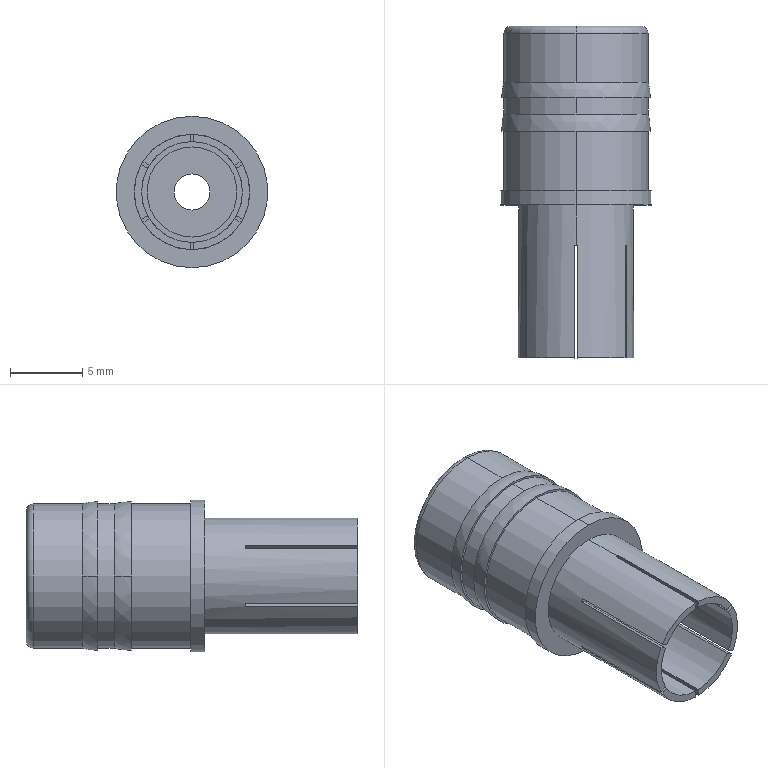Part | SolidWorks | features CirPattern 1, Fillet 1, ICE 1, Revolution 1 | 1 solid | 53 faces | box 10.5 x 23 x 10.5 mm | volume 736.39 mm3 | plane 31 | cylinder 16 | spline 4 | torus 2 | commonest cylinder face diameters 10 x6 2.5 x2 6.25 x2 7 x2 8 x2 10.5 x2